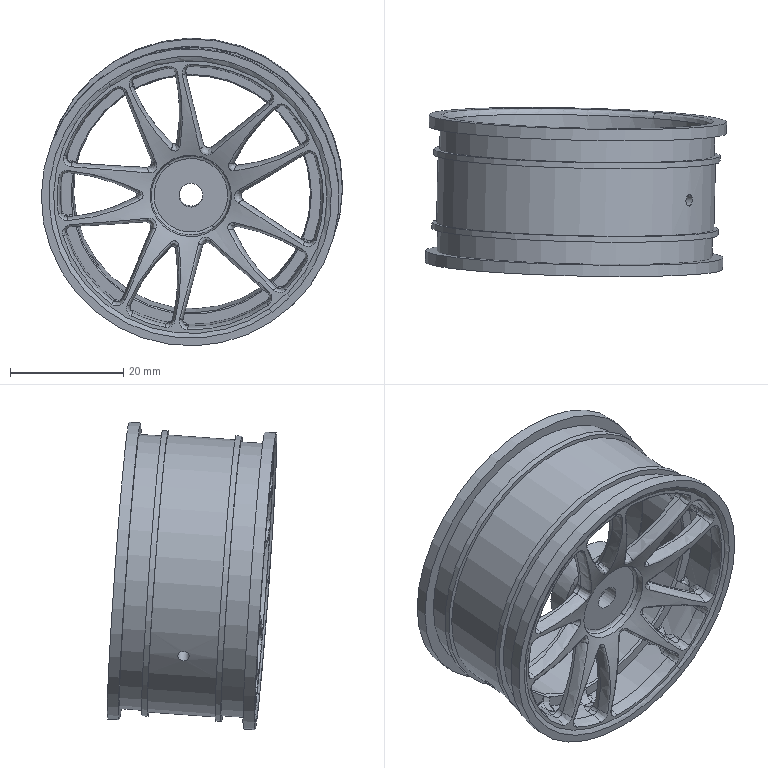Part | STEP file | jante JR29 | 1 solid | 309 faces | box 53.113 x 29.9 x 54.23 mm | volume 11757 mm3 | spline 140 | cylinder 109 | plane 58 | other 1 | cone 1 | commonest cylinder face diameters 2 x61 60 x20 46 x11 1 x7 48.5 x2 50.5 x2